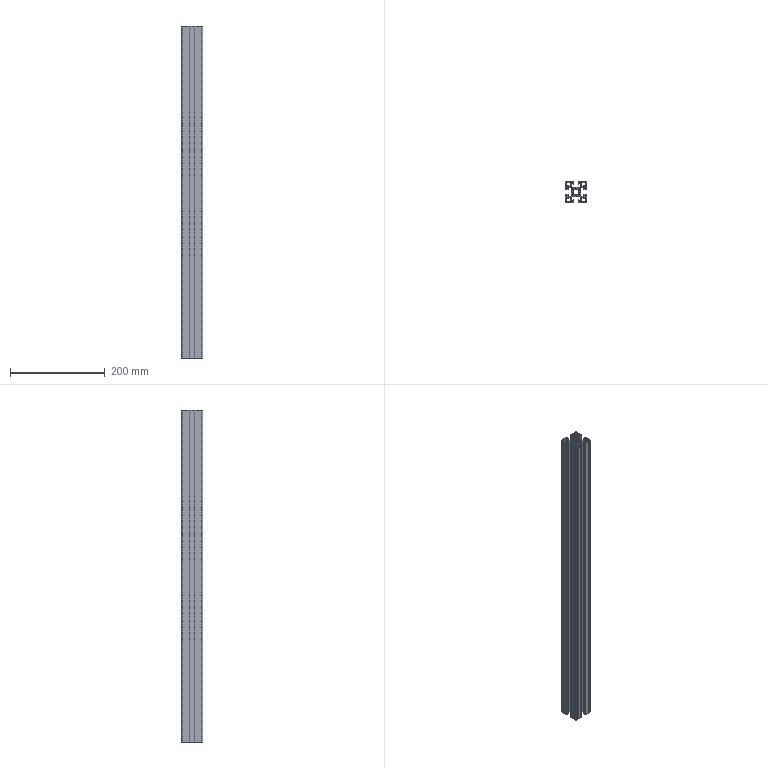Part | SolidWorks | features Extrusion 1 | 1 solid | 236 faces | box 45 x 45 x 700 mm | volume 446684 mm3 | plane 178 | cylinder 58 | commonest cylinder face diameters 2 x36 3 x10 12 x8 4 x4